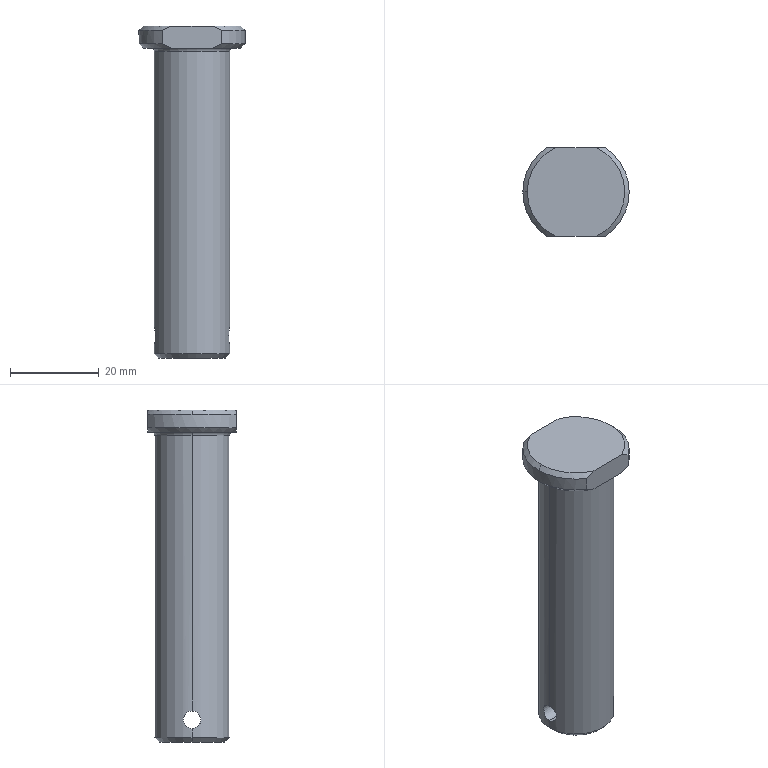Part | SolidWorks | features ICE 2, Fillet 1, Revolution 1 | 1 solid | 22 faces | box 24 x 20 x 75 mm | volume 17692 mm3 | cone 8 | cylinder 7 | plane 5 | torus 2 | commonest cylinder face diameters 24 x3 4 x2 17 x2
STEP:
#1=CARTESIAN_POINT('',(-9.3,0.,-5.));
#2=VERTEX_POINT('',#1);
#3=CARTESIAN_POINT('',(9.3,0.,-5.));
#4=VERTEX_POINT('',#3);
#5=CARTESIAN_POINT('',(0.,0.,-5.));
#6=DIRECTION('',(0.,0.,1.));
#7=DIRECTION('',(1.,0.,0.));
#8=AXIS2_PLACEMENT_3D('',#5,#6,#7);
#9=CIRCLE('',#8,9.3);
#10=EDGE_CURVE('',#2,#4,#9,.T.);
#11=ORIENTED_EDGE('',*,*,#10,.F.);
#12=CARTESIAN_POINT('',(-8.5,0.,-5.8));
#13=VERTEX_POINT('',#12);
#14=CARTESIAN_POINT('',(-9.3,0.,-5.8));
#15=DIRECTION('',(0.,1.,0.));
#16=DIRECTION('',(-1.,0.,0.));
#17=AXIS2_PLACEMENT_3D('',#14,#15,#16);
#18=CIRCLE('',#17,0.8);
#19=EDGE_CURVE('',#2,#13,#18,.T.);
#20=ORIENTED_EDGE('',*,*,#19,.T.);
#21=CARTESIAN_POINT('',(8.5,0.,-5.8));
#22=VERTEX_POINT('',#21);
#23=CARTESIAN_POINT('',(0.,0.,-5.8));
#24=DIRECTION('',(0.,0.,-1.));
#25=DIRECTION('',(1.,0.,0.));
#26=AXIS2_PLACEMENT_3D('',#23,#24,#25);
#27=CIRCLE('',#26,8.5);
#28=EDGE_CURVE('',#22,#13,#27,.T.);
#29=ORIENTED_EDGE('',*,*,#28,.F.);
#30=CARTESIAN_POINT('',(9.3,0.,-5.8));
#31=DIRECTION('',(0.,-1.,0.));
#32=DIRECTION('',(0.,0.,-1.));
#33=AXIS2_PLACEMENT_3D('',#30,#31,#32);
#34=CIRCLE('',#33,0.8);
#35=EDGE_CURVE('',#4,#22,#34,.T.);
#36=ORIENTED_EDGE('',*,*,#35,.F.);
#37=EDGE_LOOP('',(#11,#20,#29,#36));
#38=FACE_OUTER_BOUND('',#37,.T.);
#39=CARTESIAN_POINT('',(0.,0.,-5.8));
#40=DIRECTION('',(0.,0.,1.));
#41=DIRECTION('',(1.,0.,0.));
#42=AXIS2_PLACEMENT_3D('',#39,#40,#41);
#43=TOROIDAL_SURFACE('',#42,9.3,0.8);
#44=ADVANCED_FACE('',(#38),#43,.F.);
#45=CARTESIAN_POINT('',(-8.5,0.,-72.));
#46=VERTEX_POINT('',#45);
#47=CARTESIAN_POINT('',(-8.5,0.,-68.));
#48=VERTEX_POINT('',#47);
#49=CARTESIAN_POINT('',(-8.5,0.,-72.));
#50=CARTESIAN_POINT('',(-8.5,-0.1326,-72.));
#51=CARTESIAN_POINT('',(-8.497,-0.263,-71.987));
#52=CARTESIAN_POINT('',(-8.485,-0.5193,-71.936));
#53=CARTESIAN_POINT('',(-8.476,-0.6466,-71.897));
#54=CARTESIAN_POINT('',(-8.454,-0.8886,-71.797));
#55=CARTESIAN_POINT('',(-8.441,-1.003,-71.735));
#56=CARTESIAN_POINT('',(-8.413,-1.22,-71.59));
#57=CARTESIAN_POINT('',(-8.397,-1.323,-71.506));
#58=CARTESIAN_POINT('',(-8.35,-1.598,-71.23));
#59=CARTESIAN_POINT('',(-8.319,-1.747,-71.008));
#60=CARTESIAN_POINT('',(-8.286,-1.897,-70.647));
#61=CARTESIAN_POINT('',(-8.277,-1.936,-70.52));
#62=CARTESIAN_POINT('',(-8.264,-1.987,-70.262));
#63=CARTESIAN_POINT('',(-8.261,-2.,-70.132));
#64=CARTESIAN_POINT('',(-8.261,-2.,-69.87));
#65=CARTESIAN_POINT('',(-8.265,-1.987,-69.737));
#66=CARTESIAN_POINT('',(-8.277,-1.936,-69.48));
#67=CARTESIAN_POINT('',(-8.286,-1.898,-69.355));
#68=CARTESIAN_POINT('',(-8.319,-1.747,-68.991));
#69=CARTESIAN_POINT('',(-8.35,-1.599,-68.771));
#70=CARTESIAN_POINT('',(-8.397,-1.321,-68.493));
#71=CARTESIAN_POINT('',(-8.413,-1.221,-68.41));
#72=CARTESIAN_POINT('',(-8.441,-1.004,-68.266));
#73=CARTESIAN_POINT('',(-8.454,-0.8873,-68.203));
#74=CARTESIAN_POINT('',(-8.476,-0.6457,-68.103));
#75=CARTESIAN_POINT('',(-8.485,-0.521,-68.065));
#76=CARTESIAN_POINT('',(-8.497,-0.2636,-68.013));
#77=CARTESIAN_POINT('',(-8.5,-0.1308,-68.));
#78=CARTESIAN_POINT('',(-8.5,0.,-68.));
#79=B_SPLINE_CURVE_WITH_KNOTS('',3,(#49,#50,#51,#52,#53,#54,#55,#56,#57,#58,#59,#60,#61,#62,#63,#64,#65,#66,#67,#68,#69,#70,#71,#72,#73,#74,#75,#76,#77,#78),.UNSPECIFIED.,.F.,.F.,(4,2,2,2,2,2,2,2,2,2,2,2,2,2,4),(0.,0.0003922,0.0007844,0.001177,0.001569,0.002353,0.002745,0.003137,0.00353,0.003922,0.004706,0.005098,0.005491,0.005883,0.006275),.UNSPECIFIED.);
#80=EDGE_CURVE('',#46,#48,#79,.T.);
#81=ORIENTED_EDGE('',*,*,#80,.T.);
#82=CARTESIAN_POINT('',(8.5,0.,-68.));
#83=VERTEX_POINT('',#82);
#84=CARTESIAN_POINT('',(-10.,0.,-68.));
#85=DIRECTION('',(1.,0.,0.));
#86=VECTOR('',#85,1000.);
#87=LINE('',#84,#86);
#88=EDGE_CURVE('',#48,#83,#87,.T.);
#89=ORIENTED_EDGE('',*,*,#88,.T.);
#90=CARTESIAN_POINT('',(8.5,0.,-72.));
#91=VERTEX_POINT('',#90);
#92=CARTESIAN_POINT('',(8.5,0.,-68.));
#93=CARTESIAN_POINT('',(8.5,-0.2615,-68.));
#94=CARTESIAN_POINT('',(8.487,-0.5256,-68.053));
#95=CARTESIAN_POINT('',(8.454,-0.8868,-68.203));
#96=CARTESIAN_POINT('',(8.441,-1.004,-68.265));
#97=CARTESIAN_POINT('',(8.413,-1.221,-68.411));
#98=CARTESIAN_POINT('',(8.397,-1.321,-68.493));
#99=CARTESIAN_POINT('',(8.366,-1.506,-68.677));
#100=CARTESIAN_POINT('',(8.35,-1.59,-68.78));
#101=CARTESIAN_POINT('',(8.321,-1.735,-68.996));
#102=CARTESIAN_POINT('',(8.308,-1.796,-69.11));
#103=CARTESIAN_POINT('',(8.274,-1.948,-69.475));
#104=CARTESIAN_POINT('',(8.261,-2.,-69.735));
#105=CARTESIAN_POINT('',(8.261,-2.,-70.131));
#106=CARTESIAN_POINT('',(8.264,-1.987,-70.261));
#107=CARTESIAN_POINT('',(8.277,-1.936,-70.518));
#108=CARTESIAN_POINT('',(8.286,-1.897,-70.646));
#109=CARTESIAN_POINT('',(8.319,-1.747,-71.008));
#110=CARTESIAN_POINT('',(8.35,-1.599,-71.23));
#111=CARTESIAN_POINT('',(8.412,-1.232,-71.597));
#112=CARTESIAN_POINT('',(8.443,-1.009,-71.746));
#113=CARTESIAN_POINT('',(8.476,-0.6485,-71.896));
#114=CARTESIAN_POINT('',(8.485,-0.5212,-71.935));
#115=CARTESIAN_POINT('',(8.497,-0.2634,-71.987));
#116=CARTESIAN_POINT('',(8.5,-0.1326,-72.));
#117=CARTESIAN_POINT('',(8.5,0.,-72.));
#118=B_SPLINE_CURVE_WITH_KNOTS('',3,(#92,#93,#94,#95,#96,#97,#98,#99,#100,#101,#102,#103,#104,#105,#106,#107,#108,#109,#110,#111,#112,#113,#114,#115,#116,#117),.UNSPECIFIED.,.F.,.F.,(4,2,2,2,2,2,2,2,2,2,2,2,4),(0.006275,0.007059,0.007451,0.007843,0.008235,0.008627,0.009412,0.009804,0.0102,0.01098,0.01176,0.01216,0.01255),.UNSPECIFIED.);
#119=EDGE_CURVE('',#83,#91,#118,.T.);
#120=ORIENTED_EDGE('',*,*,#119,.T.);
#121=CARTESIAN_POINT('',(-10.,0.,-72.));
#122=DIRECTION('',(1.,0.,0.));
#123=VECTOR('',#122,1000.);
#124=LINE('',#121,#123);
#125=EDGE_CURVE('',#46,#91,#124,.T.);
#126=ORIENTED_EDGE('',*,*,#125,.F.);
#127=EDGE_LOOP('',(#81,#89,#120,#126));
#128=FACE_OUTER_BOUND('',#127,.T.);
#129=CARTESIAN_POINT('',(-10.,0.,-70.));
#130=DIRECTION('',(1.,0.,0.));
#131=DIRECTION('',(0.,0.,-1.));
#132=AXIS2_PLACEMENT_3D('',#129,#130,#131);
#133=CYLINDRICAL_SURFACE('',#132,2.);
#134=ADVANCED_FACE('',(#128),#133,.F.);
#135=CARTESIAN_POINT('',(8.5,0.,-74.));
#136=VERTEX_POINT('',#135);
#137=CARTESIAN_POINT('',(-8.5,0.,-74.));
#138=VERTEX_POINT('',#137);
#139=CARTESIAN_POINT('',(0.,0.,-74.));
#140=DIRECTION('',(0.,0.,1.));
#141=DIRECTION('',(1.,0.,0.));
#142=AXIS2_PLACEMENT_3D('',#139,#140,#141);
#143=CIRCLE('',#142,8.5);
#144=EDGE_CURVE('',#136,#138,#143,.T.);
#145=ORIENTED_EDGE('',*,*,#144,.T.);
#146=CARTESIAN_POINT('',(-8.5,0.,-5.));
#147=DIRECTION('',(0.,0.,1.));
#148=VECTOR('',#147,1000.);
#149=LINE('',#146,#148);
#150=EDGE_CURVE('',#138,#46,#149,.T.);
#151=ORIENTED_EDGE('',*,*,#150,.T.);
#152=CARTESIAN_POINT('',(-8.5,0.,-68.));
#153=CARTESIAN_POINT('',(-8.5,0.2615,-68.));
#154=CARTESIAN_POINT('',(-8.487,0.5256,-68.053));
#155=CARTESIAN_POINT('',(-8.454,0.8868,-68.203));
#156=CARTESIAN_POINT('',(-8.441,1.004,-68.265));
#157=CARTESIAN_POINT('',(-8.413,1.221,-68.411));
#158=CARTESIAN_POINT('',(-8.397,1.321,-68.493));
#159=CARTESIAN_POINT('',(-8.366,1.506,-68.677));
#160=CARTESIAN_POINT('',(-8.35,1.59,-68.78));
#161=CARTESIAN_POINT('',(-8.321,1.735,-68.996));
#162=CARTESIAN_POINT('',(-8.308,1.796,-69.11));
#163=CARTESIAN_POINT('',(-8.274,1.948,-69.475));
#164=CARTESIAN_POINT('',(-8.261,2.,-69.735));
#165=CARTESIAN_POINT('',(-8.261,2.,-70.131));
#166=CARTESIAN_POINT('',(-8.264,1.987,-70.261));
#167=CARTESIAN_POINT('',(-8.277,1.936,-70.518));
#168=CARTESIAN_POINT('',(-8.286,1.897,-70.646));
#169=CARTESIAN_POINT('',(-8.319,1.747,-71.008));
#170=CARTESIAN_POINT('',(-8.35,1.599,-71.23));
#171=CARTESIAN_POINT('',(-8.412,1.232,-71.597));
#172=CARTESIAN_POINT('',(-8.443,1.009,-71.746));
#173=CARTESIAN_POINT('',(-8.476,0.6485,-71.896));
#174=CARTESIAN_POINT('',(-8.485,0.5212,-71.935));
#175=CARTESIAN_POINT('',(-8.497,0.2634,-71.987));
#176=CARTESIAN_POINT('',(-8.5,0.1326,-72.));
#177=CARTESIAN_POINT('',(-8.5,0.,-72.));
#178=B_SPLINE_CURVE_WITH_KNOTS('',3,(#152,#153,#154,#155,#156,#157,#158,#159,#160,#161,#162,#163,#164,#165,#166,#167,#168,#169,#170,#171,#172,#173,#174,#175,#176,#177),.UNSPECIFIED.,.F.,.F.,(4,2,2,2,2,2,2,2,2,2,2,2,4),(0.006275,0.007059,0.007451,0.007843,0.008235,0.008627,0.009412,0.009804,0.0102,0.01098,0.01176,0.01216,0.01255),.UNSPECIFIED.);
#179=EDGE_CURVE('',#48,#46,#178,.T.);
#180=ORIENTED_EDGE('',*,*,#179,.F.);
#181=CARTESIAN_POINT('',(-8.5,0.,-5.));
#182=DIRECTION('',(0.,0.,1.));
#183=VECTOR('',#182,1000.);
#184=LINE('',#181,#183);
#185=EDGE_CURVE('',#48,#13,#184,.T.);
#186=ORIENTED_EDGE('',*,*,#185,.T.);
#187=CARTESIAN_POINT('',(0.,0.,-5.8));
#188=DIRECTION('',(0.,0.,-1.));
#189=DIRECTION('',(1.,0.,0.));
#190=AXIS2_PLACEMENT_3D('',#187,#188,#189);
#191=CIRCLE('',#190,8.5);
#192=EDGE_CURVE('',#13,#22,#191,.T.);
#193=ORIENTED_EDGE('',*,*,#192,.T.);
#194=CARTESIAN_POINT('',(8.5,0.,-5.));
#195=DIRECTION('',(0.,0.,1.));
#196=VECTOR('',#195,1000.);
#197=LINE('',#194,#196);
#198=EDGE_CURVE('',#83,#22,#197,.T.);
#199=ORIENTED_EDGE('',*,*,#198,.F.);
#200=CARTESIAN_POINT('',(8.5,0.,-72.));
#201=CARTESIAN_POINT('',(8.5,0.1326,-72.));
#202=CARTESIAN_POINT('',(8.497,0.263,-71.987));
#203=CARTESIAN_POINT('',(8.485,0.5193,-71.936));
#204=CARTESIAN_POINT('',(8.476,0.6466,-71.897));
#205=CARTESIAN_POINT('',(8.454,0.8886,-71.797));
#206=CARTESIAN_POINT('',(8.441,1.003,-71.735));
#207=CARTESIAN_POINT('',(8.413,1.22,-71.59));
#208=CARTESIAN_POINT('',(8.397,1.323,-71.506));
#209=CARTESIAN_POINT('',(8.35,1.598,-71.23));
#210=CARTESIAN_POINT('',(8.319,1.747,-71.008));
#211=CARTESIAN_POINT('',(8.286,1.897,-70.647));
#212=CARTESIAN_POINT('',(8.277,1.936,-70.52));
#213=CARTESIAN_POINT('',(8.264,1.987,-70.262));
#214=CARTESIAN_POINT('',(8.261,2.,-70.132));
#215=CARTESIAN_POINT('',(8.261,2.,-69.87));
#216=CARTESIAN_POINT('',(8.265,1.987,-69.737));
#217=CARTESIAN_POINT('',(8.277,1.936,-69.48));
#218=CARTESIAN_POINT('',(8.286,1.898,-69.355));
#219=CARTESIAN_POINT('',(8.319,1.747,-68.991));
#220=CARTESIAN_POINT('',(8.35,1.599,-68.771));
#221=CARTESIAN_POINT('',(8.397,1.321,-68.493));
#222=CARTESIAN_POINT('',(8.413,1.221,-68.41));
#223=CARTESIAN_POINT('',(8.441,1.004,-68.266));
#224=CARTESIAN_POINT('',(8.454,0.8873,-68.203));
#225=CARTESIAN_POINT('',(8.476,0.6457,-68.103));
#226=CARTESIAN_POINT('',(8.485,0.521,-68.065));
#227=CARTESIAN_POINT('',(8.497,0.2636,-68.013));
#228=CARTESIAN_POINT('',(8.5,0.1308,-68.));
#229=CARTESIAN_POINT('',(8.5,0.,-68.));
#230=B_SPLINE_CURVE_WITH_KNOTS('',3,(#200,#201,#202,#203,#204,#205,#206,#207,#208,#209,#210,#211,#212,#213,#214,#215,#216,#217,#218,#219,#220,#221,#222,#223,#224,#225,#226,#227,#228,#229),.UNSPECIFIED.,.F.,.F.,(4,2,2,2,2,2,2,2,2,2,2,2,2,2,4),(0.,0.0003922,0.0007844,0.001177,0.001569,0.002353,0.002745,0.003137,0.00353,0.003922,0.004706,0.005098,0.005491,0.005883,0.006275),.UNSPECIFIED.);
#231=EDGE_CURVE('',#91,#83,#230,.T.);
#232=ORIENTED_EDGE('',*,*,#231,.F.);
#233=CARTESIAN_POINT('',(8.5,0.,-5.));
#234=DIRECTION('',(0.,0.,1.));
#235=VECTOR('',#234,1000.);
#236=LINE('',#233,#235);
#237=EDGE_CURVE('',#136,#91,#236,.T.);
#238=ORIENTED_EDGE('',*,*,#237,.F.);
#239=EDGE_LOOP('',(#145,#151,#180,#186,#193,#199,#232,#238));
#240=FACE_OUTER_BOUND('',#239,.T.);
#241=CARTESIAN_POINT('',(0.,0.,-5.));
#242=DIRECTION('',(0.,0.,1.));
#243=DIRECTION('',(1.,0.,0.));
#244=AXIS2_PLACEMENT_3D('',#241,#242,#243);
#245=CYLINDRICAL_SURFACE('',#244,8.5);
#246=ADVANCED_FACE('',(#240),#245,.T.);
#247=CARTESIAN_POINT('',(7.5,0.,-75.));
#248=VERTEX_POINT('',#247);
#249=CARTESIAN_POINT('',(-7.5,0.,-75.));
#250=VERTEX_POINT('',#249);
#251=CARTESIAN_POINT('',(0.,0.,-75.));
#252=DIRECTION('',(0.,0.,1.));
#253=DIRECTION('',(1.,0.,0.));
#254=AXIS2_PLACEMENT_3D('',#251,#252,#253);
#255=CIRCLE('',#254,7.5);
#256=EDGE_CURVE('',#248,#250,#255,.T.);
#257=ORIENTED_EDGE('',*,*,#256,.T.);
#258=CARTESIAN_POINT('',(-8.5,0.,-74.));
#259=DIRECTION('',(-0.7071,0.,0.7071));
#260=VECTOR('',#259,1000.);
#261=LINE('',#258,#260);
#262=EDGE_CURVE('',#250,#138,#261,.T.);
#263=ORIENTED_EDGE('',*,*,#262,.T.);
#264=ORIENTED_EDGE('',*,*,#144,.F.);
#265=CARTESIAN_POINT('',(8.5,0.,-74.));
#266=DIRECTION('',(0.7071,0.,0.7071));
#267=VECTOR('',#266,1000.);
#268=LINE('',#265,#267);
#269=EDGE_CURVE('',#248,#136,#268,.T.);
#270=ORIENTED_EDGE('',*,*,#269,.F.);
#271=EDGE_LOOP('',(#257,#263,#264,#270));
#272=FACE_OUTER_BOUND('',#271,.T.);
#273=CARTESIAN_POINT('',(0.,0.,-74.));
#274=DIRECTION('',(0.,0.,1.));
#275=DIRECTION('',(1.,0.,0.));
#276=AXIS2_PLACEMENT_3D('',#273,#274,#275);
#277=CONICAL_SURFACE('',#276,8.5,0.7854);
#278=ADVANCED_FACE('',(#272),#277,.T.);
#279=CARTESIAN_POINT('',(-11.,0.,0.));
#280=VERTEX_POINT('',#279);
#281=CARTESIAN_POINT('',(-4.583,-10.,0.));
#282=VERTEX_POINT('',#281);
#283=CARTESIAN_POINT('',(0.,0.,0.));
#284=DIRECTION('',(0.,0.,1.));
#285=DIRECTION('',(1.,0.,0.));
#286=AXIS2_PLACEMENT_3D('',#283,#284,#285);
#287=CIRCLE('',#286,11.);
#288=EDGE_CURVE('',#280,#282,#287,.T.);
#289=ORIENTED_EDGE('',*,*,#288,.F.);
#290=CARTESIAN_POINT('',(-12.,0.,-1.));
#291=VERTEX_POINT('',#290);
#292=CARTESIAN_POINT('',(-11.,0.,0.));
#293=DIRECTION('',(-0.7071,0.,-0.7071));
#294=VECTOR('',#293,1000.);
#295=LINE('',#292,#294);
#296=EDGE_CURVE('',#280,#291,#295,.T.);
#297=ORIENTED_EDGE('',*,*,#296,.T.);
#298=CARTESIAN_POINT('',(-6.633,-10.,-1.));
#299=VERTEX_POINT('',#298);
#300=CARTESIAN_POINT('',(0.,0.,-1.));
#301=DIRECTION('',(0.,0.,1.));
#302=DIRECTION('',(1.,0.,0.));
#303=AXIS2_PLACEMENT_3D('',#300,#301,#302);
#304=CIRCLE('',#303,12.);
#305=EDGE_CURVE('',#291,#299,#304,.T.);
#306=ORIENTED_EDGE('',*,*,#305,.T.);
#307=CARTESIAN_POINT('',(-4.583,-10.,0.));
#308=CARTESIAN_POINT('',(-5.282,-10.,-0.2912));
#309=CARTESIAN_POINT('',(-5.966,-10.,-0.6311));
#310=CARTESIAN_POINT('',(-6.633,-10.,-1.));
#311=B_SPLINE_CURVE_WITH_KNOTS('',3,(#307,#308,#309,#310),.UNSPECIFIED.,.F.,.F.,(4,4),(0.01168,0.01394),.UNSPECIFIED.);
#312=EDGE_CURVE('',#282,#299,#311,.T.);
#313=ORIENTED_EDGE('',*,*,#312,.F.);
#314=EDGE_LOOP('',(#289,#297,#306,#313));
#315=FACE_OUTER_BOUND('',#314,.T.);
#316=CARTESIAN_POINT('',(0.,0.,0.));
#317=DIRECTION('',(0.,0.,-1.));
#318=DIRECTION('',(-1.,0.,0.));
#319=AXIS2_PLACEMENT_3D('',#316,#317,#318);
#320=CONICAL_SURFACE('',#319,11.,0.7854);
#321=ADVANCED_FACE('',(#315),#320,.T.);
#322=CARTESIAN_POINT('',(6.633,-10.,-4.));
#323=VERTEX_POINT('',#322);
#324=CARTESIAN_POINT('',(12.,0.,-4.));
#325=VERTEX_POINT('',#324);
#326=CARTESIAN_POINT('',(0.,0.,-4.));
#327=DIRECTION('',(0.,0.,1.));
#328=DIRECTION('',(1.,0.,0.));
#329=AXIS2_PLACEMENT_3D('',#326,#327,#328);
#330=CIRCLE('',#329,12.);
#331=EDGE_CURVE('',#323,#325,#330,.T.);
#332=ORIENTED_EDGE('',*,*,#331,.T.);
#333=CARTESIAN_POINT('',(12.,0.,-1.));
#334=VERTEX_POINT('',#333);
#335=CARTESIAN_POINT('',(12.,0.,-5.));
#336=DIRECTION('',(0.,0.,1.));
#337=VECTOR('',#336,1000.);
#338=LINE('',#335,#337);
#339=EDGE_CURVE('',#325,#334,#338,.T.);
#340=ORIENTED_EDGE('',*,*,#339,.T.);
#341=CARTESIAN_POINT('',(6.633,-10.,-1.));
#342=VERTEX_POINT('',#341);
#343=CARTESIAN_POINT('',(0.,0.,-1.));
#344=DIRECTION('',(0.,0.,1.));
#345=DIRECTION('',(1.,0.,0.));
#346=AXIS2_PLACEMENT_3D('',#343,#344,#345);
#347=CIRCLE('',#346,12.);
#348=EDGE_CURVE('',#342,#334,#347,.T.);
#349=ORIENTED_EDGE('',*,*,#348,.F.);
#350=CARTESIAN_POINT('',(6.633,-10.,-5.));
#351=DIRECTION('',(0.,0.,1.));
#352=VECTOR('',#351,1000.);
#353=LINE('',#350,#352);
#354=EDGE_CURVE('',#323,#342,#353,.T.);
#355=ORIENTED_EDGE('',*,*,#354,.F.);
#356=EDGE_LOOP('',(#332,#340,#349,#355));
#357=FACE_OUTER_BOUND('',#356,.T.);
#358=CARTESIAN_POINT('',(0.,0.,-5.));
#359=DIRECTION('',(0.,0.,1.));
#360=DIRECTION('',(1.,0.,0.));
#361=AXIS2_PLACEMENT_3D('',#358,#359,#360);
#362=CYLINDRICAL_SURFACE('',#361,12.);
#363=ADVANCED_FACE('',(#357),#362,.T.);
#364=CARTESIAN_POINT('',(4.583,-10.,-5.));
#365=VERTEX_POINT('',#364);
#366=CARTESIAN_POINT('',(11.,0.,-5.));
#367=VERTEX_POINT('',#366);
#368=CARTESIAN_POINT('',(0.,0.,-5.));
#369=DIRECTION('',(0.,0.,1.));
#370=DIRECTION('',(1.,0.,0.));
#371=AXIS2_PLACEMENT_3D('',#368,#369,#370);
#372=CIRCLE('',#371,11.);
#373=EDGE_CURVE('',#365,#367,#372,.T.);
#374=ORIENTED_EDGE('',*,*,#373,.T.);
#375=CARTESIAN_POINT('',(12.,0.,-4.));
#376=DIRECTION('',(0.7071,0.,0.7071));
#377=VECTOR('',#376,1000.);
#378=LINE('',#375,#377);
#379=EDGE_CURVE('',#367,#325,#378,.T.);
#380=ORIENTED_EDGE('',*,*,#379,.T.);
#381=ORIENTED_EDGE('',*,*,#331,.F.);
#382=CARTESIAN_POINT('',(4.583,-10.,-5.));
#383=CARTESIAN_POINT('',(5.282,-10.,-4.709));
#384=CARTESIAN_POINT('',(5.966,-10.,-4.369));
#385=CARTESIAN_POINT('',(6.633,-10.,-4.));
#386=B_SPLINE_CURVE_WITH_KNOTS('',3,(#382,#383,#384,#385),.UNSPECIFIED.,.F.,.F.,(4,4),(0.01168,0.01394),.UNSPECIFIED.);
#387=EDGE_CURVE('',#365,#323,#386,.T.);
#388=ORIENTED_EDGE('',*,*,#387,.F.);
#389=EDGE_LOOP('',(#374,#380,#381,#388));
#390=FACE_OUTER_BOUND('',#389,.T.);
#391=CARTESIAN_POINT('',(0.,0.,-4.));
#392=DIRECTION('',(0.,0.,1.));
#393=DIRECTION('',(1.,0.,0.));
#394=AXIS2_PLACEMENT_3D('',#391,#392,#393);
#395=CONICAL_SURFACE('',#394,12.,0.7854);
#396=ADVANCED_FACE('',(#390),#395,.T.);
#397=ORIENTED_EDGE('',*,*,#379,.F.);
#398=CARTESIAN_POINT('',(4.583,10.,-5.));
#399=VERTEX_POINT('',#398);
#400=CARTESIAN_POINT('',(0.,0.,-5.));
#401=DIRECTION('',(0.,0.,1.));
#402=DIRECTION('',(1.,0.,0.));
#403=AXIS2_PLACEMENT_3D('',#400,#401,#402);
#404=CIRCLE('',#403,11.);
#405=EDGE_CURVE('',#367,#399,#404,.T.);
#406=ORIENTED_EDGE('',*,*,#405,.T.);
#407=CARTESIAN_POINT('',(6.633,10.,-4.));
#408=VERTEX_POINT('',#407);
#409=CARTESIAN_POINT('',(6.633,10.,-4.));
#410=CARTESIAN_POINT('',(5.964,10.,-4.37));
#411=CARTESIAN_POINT('',(5.283,10.,-4.708));
#412=CARTESIAN_POINT('',(4.583,10.,-5.));
#413=B_SPLINE_CURVE_WITH_KNOTS('',3,(#409,#410,#411,#412),.UNSPECIFIED.,.F.,.F.,(4,4),(0.000001434,0.002276),.UNSPECIFIED.);
#414=EDGE_CURVE('',#408,#399,#413,.T.);
#415=ORIENTED_EDGE('',*,*,#414,.F.);
#416=CARTESIAN_POINT('',(0.,0.,-4.));
#417=DIRECTION('',(0.,0.,1.));
#418=DIRECTION('',(1.,0.,0.));
#419=AXIS2_PLACEMENT_3D('',#416,#417,#418);
#420=CIRCLE('',#419,12.);
#421=EDGE_CURVE('',#325,#408,#420,.T.);
#422=ORIENTED_EDGE('',*,*,#421,.F.);
#423=EDGE_LOOP('',(#397,#406,#415,#422));
#424=FACE_OUTER_BOUND('',#423,.T.);
#425=CARTESIAN_POINT('',(0.,0.,-4.));
#426=DIRECTION('',(0.,0.,1.));
#427=DIRECTION('',(1.,0.,0.));
#428=AXIS2_PLACEMENT_3D('',#425,#426,#427);
#429=CONICAL_SURFACE('',#428,12.,0.7854);
#430=ADVANCED_FACE('',(#424),#429,.T.);
#431=ORIENTED_EDGE('',*,*,#339,.F.);
#432=ORIENTED_EDGE('',*,*,#421,.T.);
#433=CARTESIAN_POINT('',(6.633,10.,-1.));
#434=VERTEX_POINT('',#433);
#435=CARTESIAN_POINT('',(6.633,10.,-5.));
#436=DIRECTION('',(0.,0.,-1.));
#437=VECTOR('',#436,1000.);
#438=LINE('',#435,#437);
#439=EDGE_CURVE('',#434,#408,#438,.T.);
#440=ORIENTED_EDGE('',*,*,#439,.F.);
#441=CARTESIAN_POINT('',(0.,0.,-1.));
#442=DIRECTION('',(0.,0.,1.));
#443=DIRECTION('',(1.,0.,0.));
#444=AXIS2_PLACEMENT_3D('',#441,#442,#443);
#445=CIRCLE('',#444,12.);
#446=EDGE_CURVE('',#334,#434,#445,.T.);
#447=ORIENTED_EDGE('',*,*,#446,.F.);
#448=EDGE_LOOP('',(#431,#432,#440,#447));
#449=FACE_OUTER_BOUND('',#448,.T.);
#450=CARTESIAN_POINT('',(0.,0.,-5.));
#451=DIRECTION('',(0.,0.,1.));
#452=DIRECTION('',(1.,0.,0.));
#453=AXIS2_PLACEMENT_3D('',#450,#451,#452);
#454=CYLINDRICAL_SURFACE('',#453,12.);
#455=ADVANCED_FACE('',(#449),#454,.T.);
#456=ORIENTED_EDGE('',*,*,#296,.F.);
#457=CARTESIAN_POINT('',(-4.583,10.,0.));
#458=VERTEX_POINT('',#457);
#459=CARTESIAN_POINT('',(0.,0.,0.));
#460=DIRECTION('',(0.,0.,1.));
#461=DIRECTION('',(1.,0.,0.));
#462=AXIS2_PLACEMENT_3D('',#459,#460,#461);
#463=CIRCLE('',#462,11.);
#464=EDGE_CURVE('',#458,#280,#463,.T.);
#465=ORIENTED_EDGE('',*,*,#464,.F.);
#466=CARTESIAN_POINT('',(-6.633,10.,-1.));
#467=VERTEX_POINT('',#466);
#468=CARTESIAN_POINT('',(-6.633,10.,-1.));
#469=CARTESIAN_POINT('',(-5.964,10.,-0.6301));
#470=CARTESIAN_POINT('',(-5.283,10.,-0.2916));
#471=CARTESIAN_POINT('',(-4.583,10.,0.));
#472=B_SPLINE_CURVE_WITH_KNOTS('',3,(#468,#469,#470,#471),.UNSPECIFIED.,.F.,.F.,(4,4),(0.000001434,0.002276),.UNSPECIFIED.);
#473=EDGE_CURVE('',#467,#458,#472,.T.);
#474=ORIENTED_EDGE('',*,*,#473,.F.);
#475=CARTESIAN_POINT('',(0.,0.,-1.));
#476=DIRECTION('',(0.,0.,1.));
#477=DIRECTION('',(1.,0.,0.));
#478=AXIS2_PLACEMENT_3D('',#475,#476,#477);
#479=CIRCLE('',#478,12.);
#480=EDGE_CURVE('',#467,#291,#479,.T.);
#481=ORIENTED_EDGE('',*,*,#480,.T.);
#482=EDGE_LOOP('',(#456,#465,#474,#481));
#483=FACE_OUTER_BOUND('',#482,.T.);
#484=CARTESIAN_POINT('',(0.,0.,0.));
#485=DIRECTION('',(0.,0.,-1.));
#486=DIRECTION('',(-1.,0.,0.));
#487=AXIS2_PLACEMENT_3D('',#484,#485,#486);
#488=CONICAL_SURFACE('',#487,11.,0.7854);
#489=ADVANCED_FACE('',(#483),#488,.T.);
#490=ORIENTED_EDGE('',*,*,#262,.F.);
#491=CARTESIAN_POINT('',(0.,0.,-75.));
#492=DIRECTION('',(0.,0.,1.));
#493=DIRECTION('',(1.,0.,0.));
#494=AXIS2_PLACEMENT_3D('',#491,#492,#493);
#495=CIRCLE('',#494,7.5);
#496=EDGE_CURVE('',#250,#248,#495,.T.);
#497=ORIENTED_EDGE('',*,*,#496,.T.);
#498=ORIENTED_EDGE('',*,*,#269,.T.);
#499=CARTESIAN_POINT('',(0.,0.,-74.));
#500=DIRECTION('',(0.,0.,1.));
#501=DIRECTION('',(1.,0.,0.));
#502=AXIS2_PLACEMENT_3D('',#499,#500,#501);
#503=CIRCLE('',#502,8.5);
#504=EDGE_CURVE('',#138,#136,#503,.T.);
#505=ORIENTED_EDGE('',*,*,#504,.F.);
#506=EDGE_LOOP('',(#490,#497,#498,#505));
#507=FACE_OUTER_BOUND('',#506,.T.);
#508=CARTESIAN_POINT('',(0.,0.,-74.));
#509=DIRECTION('',(0.,0.,1.));
#510=DIRECTION('',(1.,0.,0.));
#511=AXIS2_PLACEMENT_3D('',#508,#509,#510);
#512=CONICAL_SURFACE('',#511,8.5,0.7854);
#513=ADVANCED_FACE('',(#507),#512,.T.);
#514=ORIENTED_EDGE('',*,*,#150,.F.);
#515=ORIENTED_EDGE('',*,*,#504,.T.);
#516=ORIENTED_EDGE('',*,*,#237,.T.);
#517=ORIENTED_EDGE('',*,*,#119,.F.);
#518=ORIENTED_EDGE('',*,*,#198,.T.);
#519=ORIENTED_EDGE('',*,*,#28,.T.);
#520=ORIENTED_EDGE('',*,*,#185,.F.);
#521=ORIENTED_EDGE('',*,*,#80,.F.);
#522=EDGE_LOOP('',(#514,#515,#516,#517,#518,#519,#520,#521));
#523=FACE_OUTER_BOUND('',#522,.T.);
#524=CARTESIAN_POINT('',(0.,0.,-5.));
#525=DIRECTION('',(0.,0.,1.));
#526=DIRECTION('',(1.,0.,0.));
#527=AXIS2_PLACEMENT_3D('',#524,#525,#526);
#528=CYLINDRICAL_SURFACE('',#527,8.5);
#529=ADVANCED_FACE('',(#523),#528,.T.);
#530=CARTESIAN_POINT('',(0.,0.,-5.));
#531=DIRECTION('',(0.,0.,1.));
#532=DIRECTION('',(1.,0.,0.));
#533=AXIS2_PLACEMENT_3D('',#530,#531,#532);
#534=CIRCLE('',#533,9.3);
#535=EDGE_CURVE('',#4,#2,#534,.T.);
#536=ORIENTED_EDGE('',*,*,#535,.T.);
#537=ORIENTED_EDGE('',*,*,#10,.T.);
#538=EDGE_LOOP('',(#536,#537));
#539=FACE_BOUND('',#538,.T.);
#540=CARTESIAN_POINT('',(-4.583,10.,-5.));
#541=VERTEX_POINT('',#540);
#542=CARTESIAN_POINT('',(-4.583,-10.,-5.));
#543=VERTEX_POINT('',#542);
#544=CARTESIAN_POINT('',(0.,0.,-5.));
#545=DIRECTION('',(0.,0.,1.));
#546=DIRECTION('',(1.,0.,0.));
#547=AXIS2_PLACEMENT_3D('',#544,#545,#546);
#548=CIRCLE('',#547,11.);
#549=EDGE_CURVE('',#541,#543,#548,.T.);
#550=ORIENTED_EDGE('',*,*,#549,.F.);
#551=CARTESIAN_POINT('',(-14.281,10.,-5.));
#552=DIRECTION('',(1.,0.,0.));
#553=VECTOR('',#552,1000.);
#554=LINE('',#551,#553);
#555=EDGE_CURVE('',#541,#399,#554,.T.);
#556=ORIENTED_EDGE('',*,*,#555,.T.);
#557=ORIENTED_EDGE('',*,*,#405,.F.);
#558=ORIENTED_EDGE('',*,*,#373,.F.);
#559=CARTESIAN_POINT('',(-12.767,-10.,-5.));
#560=DIRECTION('',(-1.,0.,0.));
#561=VECTOR('',#560,1000.);
#562=LINE('',#559,#561);
#563=EDGE_CURVE('',#365,#543,#562,.T.);
#564=ORIENTED_EDGE('',*,*,#563,.T.);
#565=EDGE_LOOP('',(#550,#556,#557,#558,#564));
#566=FACE_OUTER_BOUND('',#565,.T.);
#567=CARTESIAN_POINT('',(0.,0.,-5.));
#568=DIRECTION('',(0.,0.,1.));
#569=DIRECTION('',(1.,0.,0.));
#570=AXIS2_PLACEMENT_3D('',#567,#568,#569);
#571=PLANE('',#570);
#572=ADVANCED_FACE('',(#539,#566),#571,.F.);
#573=CARTESIAN_POINT('',(-6.633,10.,-4.));
#574=VERTEX_POINT('',#573);
#575=CARTESIAN_POINT('',(-4.583,10.,-5.));
#576=CARTESIAN_POINT('',(-5.282,10.,-4.709));
#577=CARTESIAN_POINT('',(-5.966,10.,-4.369));
#578=CARTESIAN_POINT('',(-6.633,10.,-4.));
#579=B_SPLINE_CURVE_WITH_KNOTS('',3,(#575,#576,#577,#578),.UNSPECIFIED.,.F.,.F.,(4,4),(0.01168,0.01394),.UNSPECIFIED.);
#580=EDGE_CURVE('',#541,#574,#579,.T.);
#581=ORIENTED_EDGE('',*,*,#580,.F.);
#582=ORIENTED_EDGE('',*,*,#549,.T.);
#583=CARTESIAN_POINT('',(-6.633,-10.,-4.));
#584=VERTEX_POINT('',#583);
#585=CARTESIAN_POINT('',(-6.633,-10.,-4.));
#586=CARTESIAN_POINT('',(-5.964,-10.,-4.37));
#587=CARTESIAN_POINT('',(-5.283,-10.,-4.708));
#588=CARTESIAN_POINT('',(-4.583,-10.,-5.));
#589=B_SPLINE_CURVE_WITH_KNOTS('',3,(#585,#586,#587,#588),.UNSPECIFIED.,.F.,.F.,(4,4),(0.000001434,0.002276),.UNSPECIFIED.);
#590=EDGE_CURVE('',#584,#543,#589,.T.);
#591=ORIENTED_EDGE('',*,*,#590,.F.);
#592=CARTESIAN_POINT('',(0.,0.,-4.));
#593=DIRECTION('',(0.,0.,1.));
#594=DIRECTION('',(1.,0.,0.));
#595=AXIS2_PLACEMENT_3D('',#592,#593,#594);
#596=CIRCLE('',#595,12.);
#597=EDGE_CURVE('',#574,#584,#596,.T.);
#598=ORIENTED_EDGE('',*,*,#597,.F.);
#599=EDGE_LOOP('',(#581,#582,#591,#598));
#600=FACE_OUTER_BOUND('',#599,.T.);
#601=CARTESIAN_POINT('',(0.,0.,-4.));
#602=DIRECTION('',(0.,0.,1.));
#603=DIRECTION('',(1.,0.,0.));
#604=AXIS2_PLACEMENT_3D('',#601,#602,#603);
#605=CONICAL_SURFACE('',#604,12.,0.7854);
#606=ADVANCED_FACE('',(#600),#605,.T.);
#607=CARTESIAN_POINT('',(-6.633,10.,-5.));
#608=DIRECTION('',(0.,0.,1.));
#609=VECTOR('',#608,1000.);
#610=LINE('',#607,#609);
#611=EDGE_CURVE('',#574,#467,#610,.T.);
#612=ORIENTED_EDGE('',*,*,#611,.F.);
#613=ORIENTED_EDGE('',*,*,#597,.T.);
#614=CARTESIAN_POINT('',(-6.633,-10.,-5.));
#615=DIRECTION('',(0.,0.,-1.));
#616=VECTOR('',#615,1000.);
#617=LINE('',#614,#616);
#618=EDGE_CURVE('',#299,#584,#617,.T.);
#619=ORIENTED_EDGE('',*,*,#618,.F.);
#620=ORIENTED_EDGE('',*,*,#305,.F.);
#621=ORIENTED_EDGE('',*,*,#480,.F.);
#622=EDGE_LOOP('',(#612,#613,#619,#620,#621));
#623=FACE_OUTER_BOUND('',#622,.T.);
#624=CARTESIAN_POINT('',(0.,0.,-5.));
#625=DIRECTION('',(0.,0.,1.));
#626=DIRECTION('',(1.,0.,0.));
#627=AXIS2_PLACEMENT_3D('',#624,#625,#626);
#628=CYLINDRICAL_SURFACE('',#627,12.);
#629=ADVANCED_FACE('',(#623),#628,.T.);
#630=CARTESIAN_POINT('',(4.583,10.,0.));
#631=VERTEX_POINT('',#630);
#632=CARTESIAN_POINT('',(4.583,10.,0.));
#633=CARTESIAN_POINT('',(5.282,10.,-0.2912));
#634=CARTESIAN_POINT('',(5.966,10.,-0.6311));
#635=CARTESIAN_POINT('',(6.633,10.,-1.));
#636=B_SPLINE_CURVE_WITH_KNOTS('',3,(#632,#633,#634,#635),.UNSPECIFIED.,.F.,.F.,(4,4),(0.01168,0.01394),.UNSPECIFIED.);
#637=EDGE_CURVE('',#631,#434,#636,.T.);
#638=ORIENTED_EDGE('',*,*,#637,.F.);
#639=CARTESIAN_POINT('',(4.583,-10.,0.));
#640=VERTEX_POINT('',#639);
#641=CARTESIAN_POINT('',(0.,0.,0.));
#642=DIRECTION('',(0.,0.,1.));
#643=DIRECTION('',(1.,0.,0.));
#644=AXIS2_PLACEMENT_3D('',#641,#642,#643);
#645=CIRCLE('',#644,11.);
#646=EDGE_CURVE('',#640,#631,#645,.T.);
#647=ORIENTED_EDGE('',*,*,#646,.F.);
#648=CARTESIAN_POINT('',(6.633,-10.,-1.));
#649=CARTESIAN_POINT('',(5.964,-10.,-0.6301));
#650=CARTESIAN_POINT('',(5.283,-10.,-0.2916));
#651=CARTESIAN_POINT('',(4.583,-10.,0.));
#652=B_SPLINE_CURVE_WITH_KNOTS('',3,(#648,#649,#650,#651),.UNSPECIFIED.,.F.,.F.,(4,4),(0.000001434,0.002276),.UNSPECIFIED.);
#653=EDGE_CURVE('',#342,#640,#652,.T.);
#654=ORIENTED_EDGE('',*,*,#653,.F.);
#655=ORIENTED_EDGE('',*,*,#348,.T.);
#656=ORIENTED_EDGE('',*,*,#446,.T.);
#657=EDGE_LOOP('',(#638,#647,#654,#655,#656));
#658=FACE_OUTER_BOUND('',#657,.T.);
#659=CARTESIAN_POINT('',(0.,0.,0.));
#660=DIRECTION('',(0.,0.,-1.));
#661=DIRECTION('',(-1.,0.,0.));
#662=AXIS2_PLACEMENT_3D('',#659,#660,#661);
#663=CONICAL_SURFACE('',#662,11.,0.7854);
#664=ADVANCED_FACE('',(#658),#663,.T.);
#665=CARTESIAN_POINT('',(0.,10.,0.));
#666=DIRECTION('',(1.,0.,0.));
#667=VECTOR('',#666,1000.);
#668=LINE('',#665,#667);
#669=EDGE_CURVE('',#458,#631,#668,.T.);
#670=ORIENTED_EDGE('',*,*,#669,.F.);
#671=ORIENTED_EDGE('',*,*,#464,.T.);
#672=ORIENTED_EDGE('',*,*,#288,.T.);
#673=CARTESIAN_POINT('',(0.,-10.,0.));
#674=DIRECTION('',(-1.,0.,0.));
#675=VECTOR('',#674,1000.);
#676=LINE('',#673,#675);
#677=EDGE_CURVE('',#640,#282,#676,.T.);
#678=ORIENTED_EDGE('',*,*,#677,.F.);
#679=ORIENTED_EDGE('',*,*,#646,.T.);
#680=EDGE_LOOP('',(#670,#671,#672,#678,#679));
#681=FACE_OUTER_BOUND('',#680,.T.);
#682=CARTESIAN_POINT('',(0.,0.,0.));
#683=DIRECTION('',(0.,0.,1.));
#684=DIRECTION('',(1.,0.,0.));
#685=AXIS2_PLACEMENT_3D('',#682,#683,#684);
#686=PLANE('',#685);
#687=ADVANCED_FACE('',(#681),#686,.T.);
#688=ORIENTED_EDGE('',*,*,#256,.F.);
#689=ORIENTED_EDGE('',*,*,#496,.F.);
#690=EDGE_LOOP('',(#688,#689));
#691=FACE_OUTER_BOUND('',#690,.T.);
#692=CARTESIAN_POINT('',(0.,0.,-75.));
#693=DIRECTION('',(0.,0.,1.));
#694=DIRECTION('',(1.,0.,0.));
#695=AXIS2_PLACEMENT_3D('',#692,#693,#694);
#696=PLANE('',#695);
#697=ADVANCED_FACE('',(#691),#696,.F.);
#698=ORIENTED_EDGE('',*,*,#88,.F.);
#699=ORIENTED_EDGE('',*,*,#179,.T.);
#700=ORIENTED_EDGE('',*,*,#125,.T.);
#701=ORIENTED_EDGE('',*,*,#231,.T.);
#702=EDGE_LOOP('',(#698,#699,#700,#701));
#703=FACE_OUTER_BOUND('',#702,.T.);
#704=CARTESIAN_POINT('',(-10.,0.,-70.));
#705=DIRECTION('',(1.,0.,0.));
#706=DIRECTION('',(0.,0.,-1.));
#707=AXIS2_PLACEMENT_3D('',#704,#705,#706);
#708=CYLINDRICAL_SURFACE('',#707,2.);
#709=ADVANCED_FACE('',(#703),#708,.F.);
#710=ORIENTED_EDGE('',*,*,#590,.T.);
#711=ORIENTED_EDGE('',*,*,#563,.F.);
#712=ORIENTED_EDGE('',*,*,#387,.T.);
#713=ORIENTED_EDGE('',*,*,#354,.T.);
#714=ORIENTED_EDGE('',*,*,#653,.T.);
#715=ORIENTED_EDGE('',*,*,#677,.T.);
#716=ORIENTED_EDGE('',*,*,#312,.T.);
#717=ORIENTED_EDGE('',*,*,#618,.T.);
#718=EDGE_LOOP('',(#710,#711,#712,#713,#714,#715,#716,#717));
#719=FACE_OUTER_BOUND('',#718,.T.);
#720=CARTESIAN_POINT('',(-12.767,-10.,-5.));
#721=DIRECTION('',(0.,1.,0.));
#722=DIRECTION('',(0.,0.,1.));
#723=AXIS2_PLACEMENT_3D('',#720,#721,#722);
#724=PLANE('',#723);
#725=ADVANCED_FACE('',(#719),#724,.F.);
#726=ORIENTED_EDGE('',*,*,#414,.T.);
#727=ORIENTED_EDGE('',*,*,#555,.F.);
#728=ORIENTED_EDGE('',*,*,#580,.T.);
#729=ORIENTED_EDGE('',*,*,#611,.T.);
#730=ORIENTED_EDGE('',*,*,#473,.T.);
#731=ORIENTED_EDGE('',*,*,#669,.T.);
#732=ORIENTED_EDGE('',*,*,#637,.T.);
#733=ORIENTED_EDGE('',*,*,#439,.T.);
#734=EDGE_LOOP('',(#726,#727,#728,#729,#730,#731,#732,#733));
#735=FACE_OUTER_BOUND('',#734,.T.);
#736=CARTESIAN_POINT('',(-14.281,10.,-5.));
#737=DIRECTION('',(0.,-1.,0.));
#738=DIRECTION('',(0.,0.,-1.));
#739=AXIS2_PLACEMENT_3D('',#736,#737,#738);
#740=PLANE('',#739);
#741=ADVANCED_FACE('',(#735),#740,.F.);
#742=ORIENTED_EDGE('',*,*,#19,.F.);
#743=ORIENTED_EDGE('',*,*,#535,.F.);
#744=ORIENTED_EDGE('',*,*,#35,.T.);
#745=ORIENTED_EDGE('',*,*,#192,.F.);
#746=EDGE_LOOP('',(#742,#743,#744,#745));
#747=FACE_OUTER_BOUND('',#746,.T.);
#748=CARTESIAN_POINT('',(0.,0.,-5.8));
#749=DIRECTION('',(0.,0.,1.));
#750=DIRECTION('',(1.,0.,0.));
#751=AXIS2_PLACEMENT_3D('',#748,#749,#750);
#752=TOROIDAL_SURFACE('',#751,9.3,0.8);
#753=ADVANCED_FACE('',(#747),#752,.F.);
#754=CLOSED_SHELL('',(#44,#134,#246,#278,#321,#363,#396,#430,#455,#489,#513,#529,#572,#606,#629,#664,#687,#697,#709,#725,#741,#753));
#755=MANIFOLD_SOLID_BREP('',#754);
#756=CARTESIAN_POINT('',(0.,0.,0.));
#757=DIRECTION('',(0.,0.,1.));
#758=DIRECTION('',(1.,0.,0.));
#759=AXIS2_PLACEMENT_3D('',#756,#757,#758);
#760=(LENGTH_UNIT()NAMED_UNIT(*)SI_UNIT(.MILLI.,.METRE.));
#761=UNCERTAINTY_MEASURE_WITH_UNIT(LENGTH_MEASURE(0.00001),#760,'','');
#762=(NAMED_UNIT(*)PLANE_ANGLE_UNIT()SI_UNIT($,.RADIAN.));
#763=(NAMED_UNIT(*)SI_UNIT($,.STERADIAN.)SOLID_ANGLE_UNIT());
#764=(GEOMETRIC_REPRESENTATION_CONTEXT(3)GLOBAL_UNCERTAINTY_ASSIGNED_CONTEXT((#761))GLOBAL_UNIT_ASSIGNED_CONTEXT((#760,#762,#763))REPRESENTATION_CONTEXT('',''));
#765=ADVANCED_BREP_SHAPE_REPRESENTATION('',(#755,#759),#764);